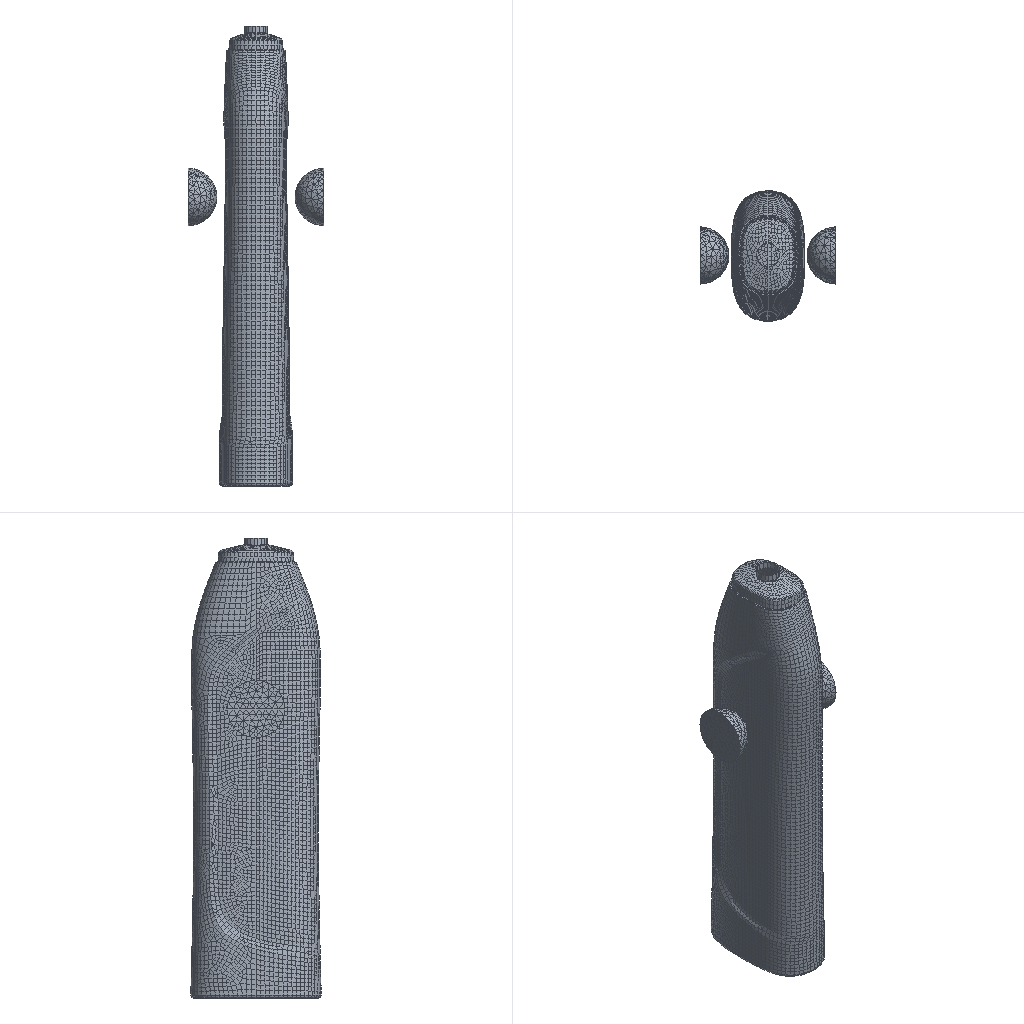Simulation study | abaqus
Set-up summary:
category,name,step,type,value,unit,region
solver,abaqus
solver,version,,,Abaqus/Standard 3DEXPERIENCE R2017x
units,not stated in the deck,,not stated
analysis,deck,,static,static
load_step,Load,Load,static,nlgeom=True
contact,interactions,,,general=0 pairs=2 ties=0
load_step,requested,,,1
mesh,nodes,,,14787
mesh,elements,,,12713
element_type,S3,,shell,104
element_type,S4R,,shell,9141
element_type,C3D10M,,solid,3468
load,load commands in deck,,count,2
bc,support commands in deck,,count,13
material,HDPE,,in results
material,PLATE,,in results
check,setup vs results,,match,"per instance, exact: element labels, types and connectivity; labels of the nodes the elements use; coordinates of those nodes at SINGLE_PRECISION in 3 of 3 instance(s)"
Abaqus input file, long lists of numbers shortened:
*Heading
** Job name: Job-2-denghou Model name: Squeeze
** Generated by: Abaqus/CAE 2017
*Preprint, echo=NO, model=NO, history=NO, contact=NO
**
** PARTS
**
*Part, name=Bottle
*Node
      1,  -1.18397713e-06,  -8.,    321.57
      2,  -2.57340298e-06,  -8.,   317.258
** (9201 more lines like these left out)
*Element, type=S4R
 1,  1,  2, 75, 90
 2, 90, 75, 76, 89
** (9139 more lines like these left out)
*Element, type=S3
4816, 5479, 5481, 5487
4817, 5497, 5494, 5496
** (102 more lines like these left out)
*Nset, nset=All, generate
    1,  9203,     1
*Elset, elset=All, generate
    1,  9245,     1
** Section: STHMapped
*Shell Section, elset=All, material=HDPE
0.5, 5
*End Part
**
*Part, name=Sphere
*Node
      1,           0.,          20.,           0.
      2,           0.,         -20.,           0.
** (2789 more lines like these left out)
*Element, type=C3D10M
   1,  227,  228,  229,  230,  420,  419,  418,  422,  421,  423
   2,  231,  232,  233,  234,  426,  425,  424,  428,  427,  429
** (1732 more lines like these left out)
*Node
   2792,           0.,           0.,           0.
*Nset, nset=Sphere-RefPt_, internal
2792,
*Nset, nset=RefPoint
 2792,
*Nset, nset=All, generate
    1,  2791,     1
*Elset, elset=All, generate
    1,  1734,     1
** Section: Rigid
*Solid Section, elset=All, material=Plate
,
*End Part
**
**
** ASSEMBLY
**
*Assembly, name=Assembly
**
*Instance, name=Bottle-1, part=Bottle
*End Instance
**
*Instance, name=Sphere-1, part=Sphere
   47.31,           0.,   202.053
   47.31,           0.,   202.053,    47.31,           1.,   202.053,          90.
*End Instance
**
*Instance, name=Sphere-2, part=Sphere
  -47.31,           0.,   202.053
  -47.31,           0.,   202.053,   -47.31,          -1.,   202.053,          90.
*End Instance
**
*Nset, nset=Fix, instance=Bottle-1
   1,   2,   3,   4,  75,  76,  77,  78,  79,  80,  81,  82,  83,  84,  85,  86
  87,  88,  89,  90, 101, 102, 103, 104, 105, 106, 107, 108, 109, 110, 111, 112
** (1 more lines like these left out)
*Elset, elset=Fix, instance=Bottle-1
  1,  2,  3,  4,  5,  6,  7,  8,  9, 28, 29, 30, 31, 32, 33, 34
 35, 36
*Nset, nset=Reaction, instance=Sphere-1
 2792,
*Nset, nset=Reaction, instance=Sphere-2
 2792,
*Nset, nset=Set-5, instance=Sphere-1
 2792,
*Nset, nset=Set-6, instance=Sphere-2
 2792,
*Elset, elset=_m_Surf-1_S3, internal, instance=Sphere-2
   38,   86,  109,  207,  211,  213,  218,  314,  316,  317,  326,  344,  351,  365,  372,  405
  411,  418,  422,  444,  446,  453,  462,  466,  473,  479,  492,  501,  543,  544,  559,  563
** (15 more lines like these left out)
*Elset, elset=_m_Surf-1_S4, internal, instance=Sphere-2
  282,  329,  500,  541,  658, 1052, 1127, 1300, 1392, 1408, 1516, 1520, 1550, 1559, 1605, 1623
*Elset, elset=_m_Surf-1_S2, internal, instance=Sphere-2
  380,  451,  788,  850, 1028, 1102, 1208, 1242, 1266, 1312, 1429, 1443, 1489, 1548, 1591, 1620
 1652, 1709, 1712
*Elset, elset=_m_Surf-1_S1, internal, instance=Sphere-2
  450,  662,  748, 1198, 1292, 1327, 1373, 1428, 1450, 1613, 1689, 1694, 1718
*Surface, type=ELEMENT, name=m_Surf-1
_m_Surf-1_S3, S3
_m_Surf-1_S4, S4
_m_Surf-1_S2, S2
_m_Surf-1_S1, S1
*Elset, elset=_m_Surf-3_S3, internal, instance=Sphere-1
   38,   86,  109,  207,  211,  213,  218,  314,  316,  317,  326,  344,  351,  365,  372,  405
  411,  418,  422,  444,  446,  453,  462,  466,  473,  479,  492,  501,  543,  544,  559,  563
** (15 more lines like these left out)
*Elset, elset=_m_Surf-3_S4, internal, instance=Sphere-1
  282,  329,  500,  541,  658, 1052, 1127, 1300, 1392, 1408, 1516, 1520, 1550, 1559, 1605, 1623
*Elset, elset=_m_Surf-3_S2, internal, instance=Sphere-1
  380,  451,  788,  850, 1028, 1102, 1208, 1242, 1266, 1312, 1429, 1443, 1489, 1548, 1591, 1620
 1652, 1709, 1712
*Elset, elset=_m_Surf-3_S1, internal, instance=Sphere-1
  450,  662,  748, 1198, 1292, 1327, 1373, 1428, 1450, 1613, 1689, 1694, 1718
*Surface, type=ELEMENT, name=m_Surf-3
_m_Surf-3_S3, S3
_m_Surf-3_S4, S4
_m_Surf-3_S2, S2
_m_Surf-3_S1, S1
*Elset, elset=_s_Surf-1_SPOS, internal, instance=Bottle-1
 1045, 1046, 1047, 1048, 1049, 1050, 1051, 1052, 1053, 1054, 1055, 1056, 1057, 1058, 1059, 1060
 1061, 1062, 1063, 1064, 1065, 1066, 1067, 1068, 1069, 1070, 1071, 1072, 1073, 1074, 1075, 1076
** (93 more lines like these left out)
*Surface, type=ELEMENT, name=s_Surf-1
_s_Surf-1_SPOS, SPOS
*Elset, elset=_s_Surf-3_SPOS, internal, instance=Bottle-1
 2177, 2178, 2179, 2180, 2181, 2182, 2183, 2184, 2185, 2186, 2187, 2188, 2189, 2190, 2191, 2192
 2193, 2194, 2195, 2196, 2197, 2198, 2199, 2200, 2201, 2202, 2203, 2204, 2205, 2206, 2207, 2208
** (98 more lines like these left out)
*Surface, type=ELEMENT, name=s_Surf-3
_s_Surf-3_SPOS, SPOS
** Constraint: Sphere-1
*Rigid Body, ref node=Sphere-1.RefPoint, elset=Sphere-1.All
** Constraint: Sphere-2
*Rigid Body, ref node=Sphere-2.RefPoint, elset=Sphere-2.All
*End Assembly
**
** MATERIALS
**
*Material, name=HDPE
*Density
 8.76e-10,
*Elastic
 903.114, 0.39
*Plastic
  8.618,    0.
 13.064, 0.007
 16.787, 0.025
 18.476, 0.044
 20.337, 0.081
 24.543,  0.28
 26.887,  0.59
*Material, name=Plate
*Density
 1.01e-06,
*Elastic
 1e+06, 0.35
**
** INTERACTION PROPERTIES
**
*Surface Interaction, name=Friction
1.,
*Friction, slip tolerance=0.005
 0.3,
**
** BOUNDARY CONDITIONS
**
** Name: FixBottle Type: Symmetry/Antisymmetry/Encastre
*Boundary
Fix, ENCASTRE
**
** INTERACTIONS
**
** Interaction: Int-2
*Contact Pair, interaction=Friction, type=SURFACE TO SURFACE
s_Surf-1, m_Surf-1
** Interaction: Int-3
*Contact Pair, interaction=Friction, type=SURFACE TO SURFACE
s_Surf-3, m_Surf-3
** ----------------------------------------------------------------
**
** STEP: Load
**
*Step, name=Load, nlgeom=YES, inc=1000
*Static
0.1, 1., 1e-05, 1.
**
** BOUNDARY CONDITIONS
**
** Name: Sphere-1 Type: Displacement/Rotation
*Boundary
Sphere-1.RefPoint, 1, 1, -18.
Sphere-1.RefPoint, 2, 2
Sphere-1.RefPoint, 3, 3
Sphere-1.RefPoint, 4, 4
Sphere-1.RefPoint, 5, 5
Sphere-1.RefPoint, 6, 6
** Name: Sphere-2 Type: Displacement/Rotation
*Boundary
Sphere-2.RefPoint, 1, 1, 18.
Sphere-2.RefPoint, 2, 2
Sphere-2.RefPoint, 3, 3
Sphere-2.RefPoint, 4, 4
Sphere-2.RefPoint, 5, 5
Sphere-2.RefPoint, 6, 6
**
** OUTPUT REQUESTS
**
*Restart, write, frequency=0
**
** FIELD OUTPUT: F-Output-1
**
*Output, field, variable=PRESELECT
**
** HISTORY OUTPUT: H-Output-1
**
*Output, history, variable=PRESELECT
*End Step
Results summary:
result,step,,completed,increments=19 time=1.0/1.0
result,analysis,,,static
result,last_loadstep,,,1
result,analysis steps,,count,1
result,primary field,,,"U, UR"
result,reaction total,,FX,-0.0,model units
result,reaction total,,FY,7e-06,model units
result,reaction total,,FZ,-1e-06,model units